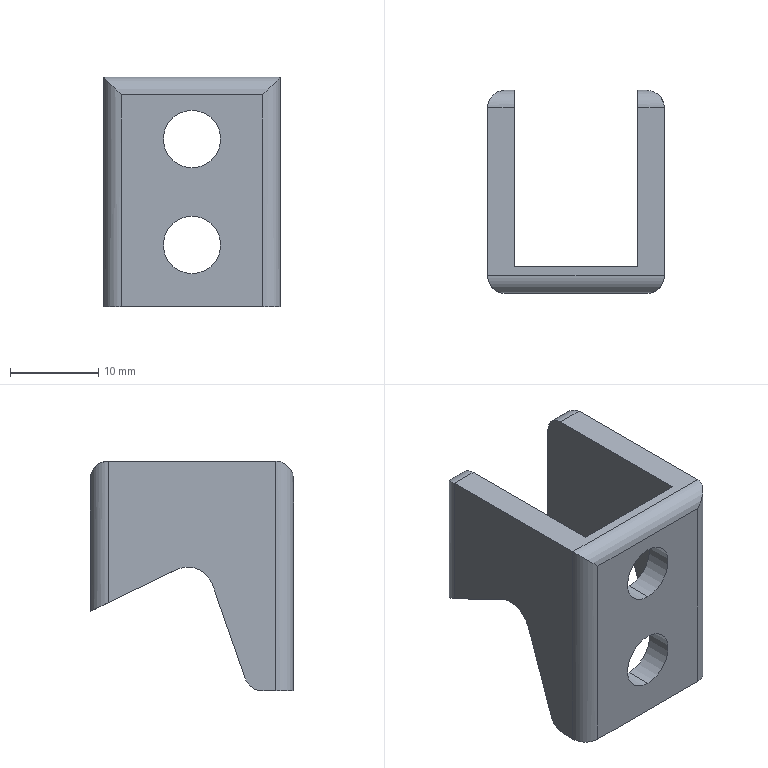Part | SolidWorks | features ICE 2, Extrusion 1, Fillet 1 | 1 solid | 31 faces | box 20 x 23 x 26 mm | volume 3238 mm3 | cylinder 17 | plane 14 | commonest cylinder face diameters 4 x9 6 x4 6.5 x4
STEP:
#1=CARTESIAN_POINT('',(0.,3.,-22.25));
#2=VERTEX_POINT('',#1);
#3=CARTESIAN_POINT('',(0.,3.,-15.75));
#4=VERTEX_POINT('',#3);
#5=CARTESIAN_POINT('',(0.,3.,-19.));
#6=DIRECTION('',(0.,1.,0.));
#7=DIRECTION('',(0.,0.,-1.));
#8=AXIS2_PLACEMENT_3D('',#5,#6,#7);
#9=CIRCLE('',#8,3.25);
#10=EDGE_CURVE('',#2,#4,#9,.T.);
#11=ORIENTED_EDGE('',*,*,#10,.T.);
#12=CARTESIAN_POINT('',(0.,0.,-15.75));
#13=VERTEX_POINT('',#12);
#14=CARTESIAN_POINT('',(0.,23.001,-15.75));
#15=DIRECTION('',(0.,-1.,0.));
#16=VECTOR('',#15,1000.);
#17=LINE('',#14,#16);
#18=EDGE_CURVE('',#4,#13,#17,.T.);
#19=ORIENTED_EDGE('',*,*,#18,.T.);
#20=CARTESIAN_POINT('',(0.,0.,-22.25));
#21=VERTEX_POINT('',#20);
#22=CARTESIAN_POINT('',(0.,0.,-19.));
#23=DIRECTION('',(0.,-1.,0.));
#24=DIRECTION('',(0.,0.,-1.));
#25=AXIS2_PLACEMENT_3D('',#22,#23,#24);
#26=CIRCLE('',#25,3.25);
#27=EDGE_CURVE('',#13,#21,#26,.T.);
#28=ORIENTED_EDGE('',*,*,#27,.T.);
#29=CARTESIAN_POINT('',(0.,23.001,-22.25));
#30=DIRECTION('',(0.,-1.,0.));
#31=VECTOR('',#30,1000.);
#32=LINE('',#29,#31);
#33=EDGE_CURVE('',#2,#21,#32,.T.);
#34=ORIENTED_EDGE('',*,*,#33,.F.);
#35=EDGE_LOOP('',(#11,#19,#28,#34));
#36=FACE_OUTER_BOUND('',#35,.T.);
#37=CARTESIAN_POINT('',(0.,23.001,-19.));
#38=DIRECTION('',(0.,-1.,0.));
#39=DIRECTION('',(0.,0.,-1.));
#40=AXIS2_PLACEMENT_3D('',#37,#38,#39);
#41=CYLINDRICAL_SURFACE('',#40,3.25);
#42=ADVANCED_FACE('',(#36),#41,.F.);
#43=CARTESIAN_POINT('',(0.,3.,-10.25));
#44=VERTEX_POINT('',#43);
#45=CARTESIAN_POINT('',(0.,3.,-3.75));
#46=VERTEX_POINT('',#45);
#47=CARTESIAN_POINT('',(0.,3.,-7.));
#48=DIRECTION('',(0.,1.,0.));
#49=DIRECTION('',(0.,0.,-1.));
#50=AXIS2_PLACEMENT_3D('',#47,#48,#49);
#51=CIRCLE('',#50,3.25);
#52=EDGE_CURVE('',#44,#46,#51,.T.);
#53=ORIENTED_EDGE('',*,*,#52,.T.);
#54=CARTESIAN_POINT('',(0.,0.,-3.75));
#55=VERTEX_POINT('',#54);
#56=CARTESIAN_POINT('',(0.,23.001,-3.75));
#57=DIRECTION('',(0.,-1.,0.));
#58=VECTOR('',#57,1000.);
#59=LINE('',#56,#58);
#60=EDGE_CURVE('',#46,#55,#59,.T.);
#61=ORIENTED_EDGE('',*,*,#60,.T.);
#62=CARTESIAN_POINT('',(0.,0.,-10.25));
#63=VERTEX_POINT('',#62);
#64=CARTESIAN_POINT('',(0.,0.,-7.));
#65=DIRECTION('',(0.,-1.,0.));
#66=DIRECTION('',(0.,0.,-1.));
#67=AXIS2_PLACEMENT_3D('',#64,#65,#66);
#68=CIRCLE('',#67,3.25);
#69=EDGE_CURVE('',#55,#63,#68,.T.);
#70=ORIENTED_EDGE('',*,*,#69,.T.);
#71=CARTESIAN_POINT('',(0.,23.001,-10.25));
#72=DIRECTION('',(0.,-1.,0.));
#73=VECTOR('',#72,1000.);
#74=LINE('',#71,#73);
#75=EDGE_CURVE('',#44,#63,#74,.T.);
#76=ORIENTED_EDGE('',*,*,#75,.F.);
#77=EDGE_LOOP('',(#53,#61,#70,#76));
#78=FACE_OUTER_BOUND('',#77,.T.);
#79=CARTESIAN_POINT('',(0.,23.001,-7.));
#80=DIRECTION('',(0.,-1.,0.));
#81=DIRECTION('',(0.,0.,-1.));
#82=AXIS2_PLACEMENT_3D('',#79,#80,#81);
#83=CYLINDRICAL_SURFACE('',#82,3.25);
#84=ADVANCED_FACE('',(#78),#83,.F.);
#85=CARTESIAN_POINT('',(10.,13.309,-12.301));
#86=VERTEX_POINT('',#85);
#87=CARTESIAN_POINT('',(10.,12.,-12.));
#88=VERTEX_POINT('',#87);
#89=CARTESIAN_POINT('',(10.,12.,-15.));
#90=DIRECTION('',(1.,0.,0.));
#91=DIRECTION('',(0.,0.,-1.));
#92=AXIS2_PLACEMENT_3D('',#89,#90,#91);
#93=CIRCLE('',#92,3.);
#94=EDGE_CURVE('',#86,#88,#93,.T.);
#95=ORIENTED_EDGE('',*,*,#94,.T.);
#96=CARTESIAN_POINT('',(7.,12.,-12.));
#97=VERTEX_POINT('',#96);
#98=CARTESIAN_POINT('',(10.,12.,-12.));
#99=DIRECTION('',(-1.,0.,0.));
#100=VECTOR('',#99,1000.);
#101=LINE('',#98,#100);
#102=EDGE_CURVE('',#88,#97,#101,.T.);
#103=ORIENTED_EDGE('',*,*,#102,.T.);
#104=CARTESIAN_POINT('',(7.,13.309,-12.301));
#105=VERTEX_POINT('',#104);
#106=CARTESIAN_POINT('',(7.,12.,-15.));
#107=DIRECTION('',(1.,0.,0.));
#108=DIRECTION('',(0.,0.,-1.));
#109=AXIS2_PLACEMENT_3D('',#106,#107,#108);
#110=CIRCLE('',#109,3.);
#111=EDGE_CURVE('',#105,#97,#110,.T.);
#112=ORIENTED_EDGE('',*,*,#111,.F.);
#113=CARTESIAN_POINT('',(10.,13.309,-12.301));
#114=DIRECTION('',(-1.,0.,0.));
#115=VECTOR('',#114,1000.);
#116=LINE('',#113,#115);
#117=EDGE_CURVE('',#86,#105,#116,.T.);
#118=ORIENTED_EDGE('',*,*,#117,.F.);
#119=EDGE_LOOP('',(#95,#103,#112,#118));
#120=FACE_OUTER_BOUND('',#119,.T.);
#121=CARTESIAN_POINT('',(10.,12.,-15.));
#122=DIRECTION('',(-1.,0.,0.));
#123=DIRECTION('',(0.,0.,1.));
#124=AXIS2_PLACEMENT_3D('',#121,#122,#123);
#125=CYLINDRICAL_SURFACE('',#124,3.);
#126=ADVANCED_FACE('',(#120),#125,.F.);
#127=CARTESIAN_POINT('',(-7.,13.309,-12.301));
#128=VERTEX_POINT('',#127);
#129=CARTESIAN_POINT('',(-7.,12.,-12.));
#130=VERTEX_POINT('',#129);
#131=CARTESIAN_POINT('',(-7.,12.,-15.));
#132=DIRECTION('',(1.,0.,0.));
#133=DIRECTION('',(0.,0.,-1.));
#134=AXIS2_PLACEMENT_3D('',#131,#132,#133);
#135=CIRCLE('',#134,3.);
#136=EDGE_CURVE('',#128,#130,#135,.T.);
#137=ORIENTED_EDGE('',*,*,#136,.T.);
#138=CARTESIAN_POINT('',(-10.,12.,-12.));
#139=VERTEX_POINT('',#138);
#140=CARTESIAN_POINT('',(10.,12.,-12.));
#141=DIRECTION('',(-1.,0.,0.));
#142=VECTOR('',#141,1000.);
#143=LINE('',#140,#142);
#144=EDGE_CURVE('',#130,#139,#143,.T.);
#145=ORIENTED_EDGE('',*,*,#144,.T.);
#146=CARTESIAN_POINT('',(-10.,13.309,-12.301));
#147=VERTEX_POINT('',#146);
#148=CARTESIAN_POINT('',(-10.,12.,-15.));
#149=DIRECTION('',(1.,0.,0.));
#150=DIRECTION('',(0.,0.,-1.));
#151=AXIS2_PLACEMENT_3D('',#148,#149,#150);
#152=CIRCLE('',#151,3.);
#153=EDGE_CURVE('',#147,#139,#152,.T.);
#154=ORIENTED_EDGE('',*,*,#153,.F.);
#155=CARTESIAN_POINT('',(10.,13.309,-12.301));
#156=DIRECTION('',(-1.,0.,0.));
#157=VECTOR('',#156,1000.);
#158=LINE('',#155,#157);
#159=EDGE_CURVE('',#128,#147,#158,.T.);
#160=ORIENTED_EDGE('',*,*,#159,.F.);
#161=EDGE_LOOP('',(#137,#145,#154,#160));
#162=FACE_OUTER_BOUND('',#161,.T.);
#163=CARTESIAN_POINT('',(10.,12.,-15.));
#164=DIRECTION('',(-1.,0.,0.));
#165=DIRECTION('',(0.,0.,1.));
#166=AXIS2_PLACEMENT_3D('',#163,#164,#165);
#167=CYLINDRICAL_SURFACE('',#166,3.);
#168=ADVANCED_FACE('',(#162),#167,.F.);
#169=ORIENTED_EDGE('',*,*,#144,.F.);
#170=CARTESIAN_POINT('',(-7.,9.166,-14.015));
#171=VERTEX_POINT('',#170);
#172=CARTESIAN_POINT('',(-7.,12.,-15.));
#173=DIRECTION('',(1.,0.,0.));
#174=DIRECTION('',(0.,0.,-1.));
#175=AXIS2_PLACEMENT_3D('',#172,#173,#174);
#176=CIRCLE('',#175,3.);
#177=EDGE_CURVE('',#130,#171,#176,.T.);
#178=ORIENTED_EDGE('',*,*,#177,.T.);
#179=CARTESIAN_POINT('',(-10.,9.166,-14.015));
#180=VERTEX_POINT('',#179);
#181=CARTESIAN_POINT('',(10.,9.166,-14.015));
#182=DIRECTION('',(-1.,0.,0.));
#183=VECTOR('',#182,1000.);
#184=LINE('',#181,#183);
#185=EDGE_CURVE('',#171,#180,#184,.T.);
#186=ORIENTED_EDGE('',*,*,#185,.T.);
#187=CARTESIAN_POINT('',(-10.,12.,-15.));
#188=DIRECTION('',(1.,0.,0.));
#189=DIRECTION('',(0.,0.,-1.));
#190=AXIS2_PLACEMENT_3D('',#187,#188,#189);
#191=CIRCLE('',#190,3.);
#192=EDGE_CURVE('',#139,#180,#191,.T.);
#193=ORIENTED_EDGE('',*,*,#192,.F.);
#194=EDGE_LOOP('',(#169,#178,#186,#193));
#195=FACE_OUTER_BOUND('',#194,.T.);
#196=CARTESIAN_POINT('',(10.,12.,-15.));
#197=DIRECTION('',(-1.,0.,0.));
#198=DIRECTION('',(0.,0.,1.));
#199=AXIS2_PLACEMENT_3D('',#196,#197,#198);
#200=CYLINDRICAL_SURFACE('',#199,3.);
#201=ADVANCED_FACE('',(#195),#200,.F.);
#202=CARTESIAN_POINT('',(-10.,21.,-16.03));
#203=VERTEX_POINT('',#202);
#204=CARTESIAN_POINT('',(-10.,-2.295,-4.734));
#205=DIRECTION('',(0.,-0.8998,0.4363));
#206=VECTOR('',#205,1000.);
#207=LINE('',#204,#206);
#208=EDGE_CURVE('',#203,#147,#207,.T.);
#209=ORIENTED_EDGE('',*,*,#208,.F.);
#210=CARTESIAN_POINT('',(-8.,23.,-17.));
#211=VERTEX_POINT('',#210);
#212=CARTESIAN_POINT('',(-10.,21.,-16.03));
#213=CARTESIAN_POINT('',(-10.,22.172,-16.598));
#214=CARTESIAN_POINT('',(-9.172,23.,-17.));
#215=CARTESIAN_POINT('',(-8.,23.,-17.));
#216=(BOUNDED_CURVE()B_SPLINE_CURVE(3,(#212,#213,#214,#215),.UNSPECIFIED.,.F.,.T.)B_SPLINE_CURVE_WITH_KNOTS((4,4),(1.571,3.142),.UNSPECIFIED.)CURVE()GEOMETRIC_REPRESENTATION_ITEM()RATIONAL_B_SPLINE_CURVE((1.,0.8047,0.8047,1.))REPRESENTATION_ITEM(''));
#217=EDGE_CURVE('',#203,#211,#216,.T.);
#218=ORIENTED_EDGE('',*,*,#217,.T.);
#219=CARTESIAN_POINT('',(-7.,23.,-17.));
#220=VERTEX_POINT('',#219);
#221=CARTESIAN_POINT('',(10.,23.,-17.));
#222=DIRECTION('',(-1.,0.,0.));
#223=VECTOR('',#222,1000.);
#224=LINE('',#221,#223);
#225=EDGE_CURVE('',#220,#211,#224,.T.);
#226=ORIENTED_EDGE('',*,*,#225,.F.);
#227=CARTESIAN_POINT('',(-7.,-2.295,-4.734));
#228=DIRECTION('',(0.,-0.8998,0.4363));
#229=VECTOR('',#228,1000.);
#230=LINE('',#227,#229);
#231=EDGE_CURVE('',#220,#128,#230,.T.);
#232=ORIENTED_EDGE('',*,*,#231,.T.);
#233=ORIENTED_EDGE('',*,*,#159,.T.);
#234=EDGE_LOOP('',(#209,#218,#226,#232,#233));
#235=FACE_OUTER_BOUND('',#234,.T.);
#236=CARTESIAN_POINT('',(10.,-2.295,-4.734));
#237=DIRECTION('',(0.,-0.4363,-0.8998));
#238=DIRECTION('',(0.,0.8998,-0.4363));
#239=AXIS2_PLACEMENT_3D('',#236,#237,#238);
#240=PLANE('',#239);
#241=ADVANCED_FACE('',(#235),#240,.T.);
#242=ORIENTED_EDGE('',*,*,#225,.T.);
#243=CARTESIAN_POINT('',(-8.,23.,-2.));
#244=VERTEX_POINT('',#243);
#245=CARTESIAN_POINT('',(-8.,23.,0.));
#246=DIRECTION('',(0.,0.,1.));
#247=VECTOR('',#246,1000.);
#248=LINE('',#245,#247);
#249=EDGE_CURVE('',#211,#244,#248,.T.);
#250=ORIENTED_EDGE('',*,*,#249,.T.);
#251=CARTESIAN_POINT('',(-7.,23.,-2.));
#252=VERTEX_POINT('',#251);
#253=CARTESIAN_POINT('',(-7.,23.,-2.));
#254=DIRECTION('',(1.,0.,0.));
#255=VECTOR('',#254,1000.);
#256=LINE('',#253,#255);
#257=EDGE_CURVE('',#244,#252,#256,.T.);
#258=ORIENTED_EDGE('',*,*,#257,.T.);
#259=CARTESIAN_POINT('',(-7.,23.,0.));
#260=DIRECTION('',(0.,0.,1.));
#261=VECTOR('',#260,1000.);
#262=LINE('',#259,#261);
#263=EDGE_CURVE('',#220,#252,#262,.T.);
#264=ORIENTED_EDGE('',*,*,#263,.F.);
#265=EDGE_LOOP('',(#242,#250,#258,#264));
#266=FACE_OUTER_BOUND('',#265,.T.);
#267=CARTESIAN_POINT('',(10.,23.,0.));
#268=DIRECTION('',(0.,1.,0.));
#269=DIRECTION('',(0.,0.,1.));
#270=AXIS2_PLACEMENT_3D('',#267,#268,#269);
#271=PLANE('',#270);
#272=ADVANCED_FACE('',(#266),#271,.T.);
#273=CARTESIAN_POINT('',(-10.,21.,0.));
#274=VERTEX_POINT('',#273);
#275=CARTESIAN_POINT('',(-10.,2.,0.));
#276=VERTEX_POINT('',#275);
#277=CARTESIAN_POINT('',(-10.,0.,0.));
#278=DIRECTION('',(0.,-1.,0.));
#279=VECTOR('',#278,1000.);
#280=LINE('',#277,#279);
#281=EDGE_CURVE('',#274,#276,#280,.T.);
#282=ORIENTED_EDGE('',*,*,#281,.T.);
#283=CARTESIAN_POINT('',(10.,2.,0.));
#284=VERTEX_POINT('',#283);
#285=CARTESIAN_POINT('',(10.,2.,0.));
#286=DIRECTION('',(1.,0.,0.));
#287=VECTOR('',#286,1000.);
#288=LINE('',#285,#287);
#289=EDGE_CURVE('',#276,#284,#288,.T.);
#290=ORIENTED_EDGE('',*,*,#289,.T.);
#291=CARTESIAN_POINT('',(10.,21.,0.));
#292=VERTEX_POINT('',#291);
#293=CARTESIAN_POINT('',(10.,0.,0.));
#294=DIRECTION('',(0.,-1.,0.));
#295=VECTOR('',#294,1000.);
#296=LINE('',#293,#295);
#297=EDGE_CURVE('',#292,#284,#296,.T.);
#298=ORIENTED_EDGE('',*,*,#297,.F.);
#299=CARTESIAN_POINT('',(7.,21.,0.));
#300=VERTEX_POINT('',#299);
#301=CARTESIAN_POINT('',(7.,21.,0.));
#302=DIRECTION('',(-1.,0.,0.));
#303=VECTOR('',#302,1000.);
#304=LINE('',#301,#303);
#305=EDGE_CURVE('',#292,#300,#304,.T.);
#306=ORIENTED_EDGE('',*,*,#305,.T.);
#307=CARTESIAN_POINT('',(7.,3.,0.));
#308=VERTEX_POINT('',#307);
#309=CARTESIAN_POINT('',(7.,23.,0.));
#310=DIRECTION('',(0.,-1.,0.));
#311=VECTOR('',#310,1000.);
#312=LINE('',#309,#311);
#313=EDGE_CURVE('',#300,#308,#312,.T.);
#314=ORIENTED_EDGE('',*,*,#313,.T.);
#315=CARTESIAN_POINT('',(-7.,3.,0.));
#316=VERTEX_POINT('',#315);
#317=CARTESIAN_POINT('',(-7.,3.,0.));
#318=DIRECTION('',(1.,0.,0.));
#319=VECTOR('',#318,1000.);
#320=LINE('',#317,#319);
#321=EDGE_CURVE('',#316,#308,#320,.T.);
#322=ORIENTED_EDGE('',*,*,#321,.F.);
#323=CARTESIAN_POINT('',(-7.,21.,0.));
#324=VERTEX_POINT('',#323);
#325=CARTESIAN_POINT('',(-7.,23.,0.));
#326=DIRECTION('',(0.,-1.,0.));
#327=VECTOR('',#326,1000.);
#328=LINE('',#325,#327);
#329=EDGE_CURVE('',#324,#316,#328,.T.);
#330=ORIENTED_EDGE('',*,*,#329,.F.);
#331=CARTESIAN_POINT('',(-10.,21.,0.));
#332=DIRECTION('',(-1.,0.,0.));
#333=VECTOR('',#332,1000.);
#334=LINE('',#331,#333);
#335=EDGE_CURVE('',#324,#274,#334,.T.);
#336=ORIENTED_EDGE('',*,*,#335,.T.);
#337=EDGE_LOOP('',(#282,#290,#298,#306,#314,#322,#330,#336));
#338=FACE_OUTER_BOUND('',#337,.T.);
#339=CARTESIAN_POINT('',(10.,0.,0.));
#340=DIRECTION('',(0.,0.,-1.));
#341=DIRECTION('',(0.,1.,0.));
#342=AXIS2_PLACEMENT_3D('',#339,#340,#341);
#343=PLANE('',#342);
#344=ADVANCED_FACE('',(#338),#343,.F.);
#345=CARTESIAN_POINT('',(7.,3.,-26.));
#346=VERTEX_POINT('',#345);
#347=CARTESIAN_POINT('',(7.,3.578,-26.));
#348=VERTEX_POINT('',#347);
#349=CARTESIAN_POINT('',(7.,23.,-26.));
#350=DIRECTION('',(0.,1.,0.));
#351=VECTOR('',#350,1000.);
#352=LINE('',#349,#351);
#353=EDGE_CURVE('',#346,#348,#352,.T.);
#354=ORIENTED_EDGE('',*,*,#353,.T.);
#355=CARTESIAN_POINT('',(10.,3.578,-26.));
#356=VERTEX_POINT('',#355);
#357=CARTESIAN_POINT('',(10.,3.578,-26.));
#358=DIRECTION('',(1.,0.,0.));
#359=VECTOR('',#358,1000.);
#360=LINE('',#357,#359);
#361=EDGE_CURVE('',#348,#356,#360,.T.);
#362=ORIENTED_EDGE('',*,*,#361,.T.);
#363=CARTESIAN_POINT('',(10.,2.,-26.));
#364=VERTEX_POINT('',#363);
#365=CARTESIAN_POINT('',(10.,0.,-26.));
#366=DIRECTION('',(0.,1.,0.));
#367=VECTOR('',#366,1000.);
#368=LINE('',#365,#367);
#369=EDGE_CURVE('',#364,#356,#368,.T.);
#370=ORIENTED_EDGE('',*,*,#369,.F.);
#371=CARTESIAN_POINT('',(8.,0.,-26.));
#372=VERTEX_POINT('',#371);
#373=CARTESIAN_POINT('',(8.,2.,-26.));
#374=DIRECTION('',(0.,0.,-1.));
#375=DIRECTION('',(1.,0.,0.));
#376=AXIS2_PLACEMENT_3D('',#373,#374,#375);
#377=CIRCLE('',#376,2.);
#378=EDGE_CURVE('',#364,#372,#377,.T.);
#379=ORIENTED_EDGE('',*,*,#378,.T.);
#380=CARTESIAN_POINT('',(-8.,0.,-26.));
#381=VERTEX_POINT('',#380);
#382=CARTESIAN_POINT('',(10.,0.,-26.));
#383=DIRECTION('',(-1.,0.,0.));
#384=VECTOR('',#383,1000.);
#385=LINE('',#382,#384);
#386=EDGE_CURVE('',#372,#381,#385,.T.);
#387=ORIENTED_EDGE('',*,*,#386,.T.);
#388=CARTESIAN_POINT('',(-10.,2.,-26.));
#389=VERTEX_POINT('',#388);
#390=CARTESIAN_POINT('',(-8.,2.,-26.));
#391=DIRECTION('',(0.,0.,-1.));
#392=DIRECTION('',(1.,0.,0.));
#393=AXIS2_PLACEMENT_3D('',#390,#391,#392);
#394=CIRCLE('',#393,2.);
#395=EDGE_CURVE('',#381,#389,#394,.T.);
#396=ORIENTED_EDGE('',*,*,#395,.T.);
#397=CARTESIAN_POINT('',(-10.,3.578,-26.));
#398=VERTEX_POINT('',#397);
#399=CARTESIAN_POINT('',(-10.,0.,-26.));
#400=DIRECTION('',(0.,1.,0.));
#401=VECTOR('',#400,1000.);
#402=LINE('',#399,#401);
#403=EDGE_CURVE('',#389,#398,#402,.T.);
#404=ORIENTED_EDGE('',*,*,#403,.T.);
#405=CARTESIAN_POINT('',(-7.,3.578,-26.));
#406=VERTEX_POINT('',#405);
#407=CARTESIAN_POINT('',(10.,3.578,-26.));
#408=DIRECTION('',(1.,0.,0.));
#409=VECTOR('',#408,1000.);
#410=LINE('',#407,#409);
#411=EDGE_CURVE('',#398,#406,#410,.T.);
#412=ORIENTED_EDGE('',*,*,#411,.T.);
#413=CARTESIAN_POINT('',(-7.,3.,-26.));
#414=VERTEX_POINT('',#413);
#415=CARTESIAN_POINT('',(-7.,23.,-26.));
#416=DIRECTION('',(0.,1.,0.));
#417=VECTOR('',#416,1000.);
#418=LINE('',#415,#417);
#419=EDGE_CURVE('',#414,#406,#418,.T.);
#420=ORIENTED_EDGE('',*,*,#419,.F.);
#421=CARTESIAN_POINT('',(-7.,3.,-26.));
#422=DIRECTION('',(1.,0.,0.));
#423=VECTOR('',#422,1000.);
#424=LINE('',#421,#423);
#425=EDGE_CURVE('',#414,#346,#424,.T.);
#426=ORIENTED_EDGE('',*,*,#425,.T.);
#427=EDGE_LOOP('',(#354,#362,#370,#379,#387,#396,#404,#412,#420,#426));
#428=FACE_OUTER_BOUND('',#427,.T.);
#429=CARTESIAN_POINT('',(10.,0.,-26.));
#430=DIRECTION('',(0.,0.,1.));
#431=DIRECTION('',(1.,0.,0.));
#432=AXIS2_PLACEMENT_3D('',#429,#430,#431);
#433=PLANE('',#432);
#434=ADVANCED_FACE('',(#428),#433,.F.);
#435=CARTESIAN_POINT('',(-7.,5.467,-24.657));
#436=VERTEX_POINT('',#435);
#437=CARTESIAN_POINT('',(-7.,12.525,-4.354));
#438=DIRECTION('',(0.,0.3284,0.9446));
#439=VECTOR('',#438,1000.);
#440=LINE('',#437,#439);
#441=EDGE_CURVE('',#436,#171,#440,.T.);
#442=ORIENTED_EDGE('',*,*,#441,.F.);
#443=CARTESIAN_POINT('',(-10.,5.467,-24.657));
#444=VERTEX_POINT('',#443);
#445=CARTESIAN_POINT('',(10.,5.467,-24.657));
#446=DIRECTION('',(-1.,0.,0.));
#447=VECTOR('',#446,1000.);
#448=LINE('',#445,#447);
#449=EDGE_CURVE('',#436,#444,#448,.T.);
#450=ORIENTED_EDGE('',*,*,#449,.T.);
#451=CARTESIAN_POINT('',(-10.,12.525,-4.354));
#452=DIRECTION('',(0.,0.3284,0.9446));
#453=VECTOR('',#452,1000.);
#454=LINE('',#451,#453);
#455=EDGE_CURVE('',#444,#180,#454,.T.);
#456=ORIENTED_EDGE('',*,*,#455,.T.);
#457=ORIENTED_EDGE('',*,*,#185,.F.);
#458=EDGE_LOOP('',(#442,#450,#456,#457));
#459=FACE_OUTER_BOUND('',#458,.T.);
#460=CARTESIAN_POINT('',(10.,12.525,-4.354));
#461=DIRECTION('',(0.,-0.9446,0.3284));
#462=DIRECTION('',(0.,-0.3284,-0.9446));
#463=AXIS2_PLACEMENT_3D('',#460,#461,#462);
#464=PLANE('',#463);
#465=ADVANCED_FACE('',(#459),#464,.F.);
#466=ORIENTED_EDGE('',*,*,#102,.F.);
#467=CARTESIAN_POINT('',(10.,9.166,-14.015));
#468=VERTEX_POINT('',#467);
#469=CARTESIAN_POINT('',(10.,12.,-15.));
#470=DIRECTION('',(1.,0.,0.));
#471=DIRECTION('',(0.,0.,-1.));
#472=AXIS2_PLACEMENT_3D('',#469,#470,#471);
#473=CIRCLE('',#472,3.);
#474=EDGE_CURVE('',#88,#468,#473,.T.);
#475=ORIENTED_EDGE('',*,*,#474,.T.);
#476=CARTESIAN_POINT('',(7.,9.166,-14.015));
#477=VERTEX_POINT('',#476);
#478=CARTESIAN_POINT('',(10.,9.166,-14.015));
#479=DIRECTION('',(-1.,0.,0.));
#480=VECTOR('',#479,1000.);
#481=LINE('',#478,#480);
#482=EDGE_CURVE('',#468,#477,#481,.T.);
#483=ORIENTED_EDGE('',*,*,#482,.T.);
#484=CARTESIAN_POINT('',(7.,12.,-15.));
#485=DIRECTION('',(1.,0.,0.));
#486=DIRECTION('',(0.,0.,-1.));
#487=AXIS2_PLACEMENT_3D('',#484,#485,#486);
#488=CIRCLE('',#487,3.);
#489=EDGE_CURVE('',#97,#477,#488,.T.);
#490=ORIENTED_EDGE('',*,*,#489,.F.);
#491=EDGE_LOOP('',(#466,#475,#483,#490));
#492=FACE_OUTER_BOUND('',#491,.T.);
#493=CARTESIAN_POINT('',(10.,12.,-15.));
#494=DIRECTION('',(-1.,0.,0.));
#495=DIRECTION('',(0.,0.,1.));
#496=AXIS2_PLACEMENT_3D('',#493,#494,#495);
#497=CYLINDRICAL_SURFACE('',#496,3.);
#498=ADVANCED_FACE('',(#492),#497,.F.);
#499=CARTESIAN_POINT('',(8.,23.,-17.));
#500=VERTEX_POINT('',#499);
#501=CARTESIAN_POINT('',(7.,23.,-17.));
#502=VERTEX_POINT('',#501);
#503=CARTESIAN_POINT('',(10.,23.,-17.));
#504=DIRECTION('',(-1.,0.,0.));
#505=VECTOR('',#504,1000.);
#506=LINE('',#503,#505);
#507=EDGE_CURVE('',#500,#502,#506,.T.);
#508=ORIENTED_EDGE('',*,*,#507,.F.);
#509=CARTESIAN_POINT('',(10.,21.,-16.03));
#510=VERTEX_POINT('',#509);
#511=CARTESIAN_POINT('',(8.,23.,-17.));
#512=CARTESIAN_POINT('',(9.172,23.,-17.));
#513=CARTESIAN_POINT('',(10.,22.172,-16.598));
#514=CARTESIAN_POINT('',(10.,21.,-16.03));
#515=(BOUNDED_CURVE()B_SPLINE_CURVE(3,(#511,#512,#513,#514),.UNSPECIFIED.,.F.,.F.)B_SPLINE_CURVE_WITH_KNOTS((4,4),(0.,1.571),.UNSPECIFIED.)CURVE()GEOMETRIC_REPRESENTATION_ITEM()RATIONAL_B_SPLINE_CURVE((1.,0.8047,0.8047,1.))REPRESENTATION_ITEM(''));
#516=EDGE_CURVE('',#500,#510,#515,.T.);
#517=ORIENTED_EDGE('',*,*,#516,.T.);
#518=CARTESIAN_POINT('',(10.,-2.295,-4.734));
#519=DIRECTION('',(0.,-0.8998,0.4363));
#520=VECTOR('',#519,1000.);
#521=LINE('',#518,#520);
#522=EDGE_CURVE('',#510,#86,#521,.T.);
#523=ORIENTED_EDGE('',*,*,#522,.T.);
#524=ORIENTED_EDGE('',*,*,#117,.T.);
#525=CARTESIAN_POINT('',(7.,-2.295,-4.734));
#526=DIRECTION('',(0.,-0.8998,0.4363));
#527=VECTOR('',#526,1000.);
#528=LINE('',#525,#527);
#529=EDGE_CURVE('',#502,#105,#528,.T.);
#530=ORIENTED_EDGE('',*,*,#529,.F.);
#531=EDGE_LOOP('',(#508,#517,#523,#524,#530));
#532=FACE_OUTER_BOUND('',#531,.T.);
#533=CARTESIAN_POINT('',(10.,-2.295,-4.734));
#534=DIRECTION('',(0.,-0.4363,-0.8998));
#535=DIRECTION('',(0.,0.8998,-0.4363));
#536=AXIS2_PLACEMENT_3D('',#533,#534,#535);
#537=PLANE('',#536);
#538=ADVANCED_FACE('',(#532),#537,.T.);
#539=CARTESIAN_POINT('',(7.,23.,-2.));
#540=VERTEX_POINT('',#539);
#541=CARTESIAN_POINT('',(8.,23.,-2.));
#542=VERTEX_POINT('',#541);
#543=CARTESIAN_POINT('',(10.,23.,-2.));
#544=DIRECTION('',(1.,0.,0.));
#545=VECTOR('',#544,1000.);
#546=LINE('',#543,#545);
#547=EDGE_CURVE('',#540,#542,#546,.T.);
#548=ORIENTED_EDGE('',*,*,#547,.T.);
#549=CARTESIAN_POINT('',(8.,23.,0.));
#550=DIRECTION('',(0.,0.,-1.));
#551=VECTOR('',#550,1000.);
#552=LINE('',#549,#551);
#553=EDGE_CURVE('',#542,#500,#552,.T.);
#554=ORIENTED_EDGE('',*,*,#553,.T.);
#555=ORIENTED_EDGE('',*,*,#507,.T.);
#556=CARTESIAN_POINT('',(7.,23.,0.));
#557=DIRECTION('',(0.,0.,1.));
#558=VECTOR('',#557,1000.);
#559=LINE('',#556,#558);
#560=EDGE_CURVE('',#502,#540,#559,.T.);
#561=ORIENTED_EDGE('',*,*,#560,.T.);
#562=EDGE_LOOP('',(#548,#554,#555,#561));
#563=FACE_OUTER_BOUND('',#562,.T.);
#564=CARTESIAN_POINT('',(10.,23.,0.));
#565=DIRECTION('',(0.,1.,0.));
#566=DIRECTION('',(0.,0.,1.));
#567=AXIS2_PLACEMENT_3D('',#564,#565,#566);
#568=PLANE('',#567);
#569=ADVANCED_FACE('',(#563),#568,.T.);
#570=CARTESIAN_POINT('',(0.,0.,-19.));
#571=DIRECTION('',(0.,-1.,0.));
#572=DIRECTION('',(0.,0.,-1.));
#573=AXIS2_PLACEMENT_3D('',#570,#571,#572);
#574=CIRCLE('',#573,3.25);
#575=EDGE_CURVE('',#21,#13,#574,.T.);
#576=ORIENTED_EDGE('',*,*,#575,.F.);
#577=ORIENTED_EDGE('',*,*,#27,.F.);
#578=EDGE_LOOP('',(#576,#577));
#579=FACE_BOUND('',#578,.T.);
#580=CARTESIAN_POINT('',(0.,0.,-7.));
#581=DIRECTION('',(0.,-1.,0.));
#582=DIRECTION('',(0.,0.,-1.));
#583=AXIS2_PLACEMENT_3D('',#580,#581,#582);
#584=CIRCLE('',#583,3.25);
#585=EDGE_CURVE('',#63,#55,#584,.T.);
#586=ORIENTED_EDGE('',*,*,#585,.F.);
#587=ORIENTED_EDGE('',*,*,#69,.F.);
#588=EDGE_LOOP('',(#586,#587));
#589=FACE_BOUND('',#588,.T.);
#590=CARTESIAN_POINT('',(8.,0.,-2.));
#591=VERTEX_POINT('',#590);
#592=CARTESIAN_POINT('',(-8.,0.,-2.));
#593=VERTEX_POINT('',#592);
#594=CARTESIAN_POINT('',(10.,0.,-2.));
#595=DIRECTION('',(-1.,0.,0.));
#596=VECTOR('',#595,1000.);
#597=LINE('',#594,#596);
#598=EDGE_CURVE('',#591,#593,#597,.T.);
#599=ORIENTED_EDGE('',*,*,#598,.T.);
#600=CARTESIAN_POINT('',(-8.,0.,0.));
#601=DIRECTION('',(0.,0.,-1.));
#602=VECTOR('',#601,1000.);
#603=LINE('',#600,#602);
#604=EDGE_CURVE('',#593,#381,#603,.T.);
#605=ORIENTED_EDGE('',*,*,#604,.T.);
#606=ORIENTED_EDGE('',*,*,#386,.F.);
#607=CARTESIAN_POINT('',(8.,0.,0.));
#608=DIRECTION('',(0.,0.,1.));
#609=VECTOR('',#608,1000.);
#610=LINE('',#607,#609);
#611=EDGE_CURVE('',#372,#591,#610,.T.);
#612=ORIENTED_EDGE('',*,*,#611,.T.);
#613=EDGE_LOOP('',(#599,#605,#606,#612));
#614=FACE_OUTER_BOUND('',#613,.T.);
#615=CARTESIAN_POINT('',(10.,0.,0.));
#616=DIRECTION('',(0.,1.,0.));
#617=DIRECTION('',(0.,0.,1.));
#618=AXIS2_PLACEMENT_3D('',#615,#616,#617);
#619=PLANE('',#618);
#620=ADVANCED_FACE('',(#579,#589,#614),#619,.F.);
#621=CARTESIAN_POINT('',(10.,5.467,-24.657));
#622=VERTEX_POINT('',#621);
#623=CARTESIAN_POINT('',(10.,12.525,-4.354));
#624=DIRECTION('',(0.,0.3284,0.9446));
#625=VECTOR('',#624,1000.);
#626=LINE('',#623,#625);
#627=EDGE_CURVE('',#622,#468,#626,.T.);
#628=ORIENTED_EDGE('',*,*,#627,.F.);
#629=CARTESIAN_POINT('',(7.,5.467,-24.657));
#630=VERTEX_POINT('',#629);
#631=CARTESIAN_POINT('',(10.,5.467,-24.657));
#632=DIRECTION('',(-1.,0.,0.));
#633=VECTOR('',#632,1000.);
#634=LINE('',#631,#633);
#635=EDGE_CURVE('',#622,#630,#634,.T.);
#636=ORIENTED_EDGE('',*,*,#635,.T.);
#637=CARTESIAN_POINT('',(7.,12.525,-4.354));
#638=DIRECTION('',(0.,0.3284,0.9446));
#639=VECTOR('',#638,1000.);
#640=LINE('',#637,#639);
#641=EDGE_CURVE('',#630,#477,#640,.T.);
#642=ORIENTED_EDGE('',*,*,#641,.T.);
#643=ORIENTED_EDGE('',*,*,#482,.F.);
#644=EDGE_LOOP('',(#628,#636,#642,#643));
#645=FACE_OUTER_BOUND('',#644,.T.);
#646=CARTESIAN_POINT('',(10.,12.525,-4.354));
#647=DIRECTION('',(0.,-0.9446,0.3284));
#648=DIRECTION('',(0.,-0.3284,-0.9446));
#649=AXIS2_PLACEMENT_3D('',#646,#647,#648);
#650=PLANE('',#649);
#651=ADVANCED_FACE('',(#645),#650,.F.);
#652=ORIENTED_EDGE('',*,*,#369,.T.);
#653=CARTESIAN_POINT('',(10.,3.578,-24.));
#654=DIRECTION('',(1.,0.,0.));
#655=DIRECTION('',(0.,0.,-1.));
#656=AXIS2_PLACEMENT_3D('',#653,#654,#655);
#657=CIRCLE('',#656,2.);
#658=EDGE_CURVE('',#356,#622,#657,.T.);
#659=ORIENTED_EDGE('',*,*,#658,.T.);
#660=ORIENTED_EDGE('',*,*,#627,.T.);
#661=ORIENTED_EDGE('',*,*,#474,.F.);
#662=ORIENTED_EDGE('',*,*,#94,.F.);
#663=ORIENTED_EDGE('',*,*,#522,.F.);
#664=CARTESIAN_POINT('',(10.,21.,0.));
#665=DIRECTION('',(0.,0.,1.));
#666=VECTOR('',#665,1000.);
#667=LINE('',#664,#666);
#668=EDGE_CURVE('',#510,#292,#667,.T.);
#669=ORIENTED_EDGE('',*,*,#668,.T.);
#670=ORIENTED_EDGE('',*,*,#297,.T.);
#671=CARTESIAN_POINT('',(10.,2.,-26.));
#672=DIRECTION('',(0.,0.,-1.));
#673=VECTOR('',#672,1000.);
#674=LINE('',#671,#673);
#675=EDGE_CURVE('',#284,#364,#674,.T.);
#676=ORIENTED_EDGE('',*,*,#675,.T.);
#677=EDGE_LOOP('',(#652,#659,#660,#661,#662,#663,#669,#670,#676));
#678=FACE_OUTER_BOUND('',#677,.T.);
#679=CARTESIAN_POINT('',(10.,0.,0.));
#680=DIRECTION('',(1.,0.,0.));
#681=DIRECTION('',(0.,0.,-1.));
#682=AXIS2_PLACEMENT_3D('',#679,#680,#681);
#683=PLANE('',#682);
#684=ADVANCED_FACE('',(#678),#683,.T.);
#685=ORIENTED_EDGE('',*,*,#455,.F.);
#686=CARTESIAN_POINT('',(-10.,3.578,-24.));
#687=DIRECTION('',(-1.,0.,0.));
#688=DIRECTION('',(0.,0.,-1.));
#689=AXIS2_PLACEMENT_3D('',#686,#687,#688);
#690=CIRCLE('',#689,2.);
#691=EDGE_CURVE('',#444,#398,#690,.T.);
#692=ORIENTED_EDGE('',*,*,#691,.T.);
#693=ORIENTED_EDGE('',*,*,#403,.F.);
#694=CARTESIAN_POINT('',(-10.,2.,0.));
#695=DIRECTION('',(0.,0.,1.));
#696=VECTOR('',#695,1000.);
#697=LINE('',#694,#696);
#698=EDGE_CURVE('',#389,#276,#697,.T.);
#699=ORIENTED_EDGE('',*,*,#698,.T.);
#700=ORIENTED_EDGE('',*,*,#281,.F.);
#701=CARTESIAN_POINT('',(-10.,21.,-17.));
#702=DIRECTION('',(0.,0.,-1.));
#703=VECTOR('',#702,1000.);
#704=LINE('',#701,#703);
#705=EDGE_CURVE('',#274,#203,#704,.T.);
#706=ORIENTED_EDGE('',*,*,#705,.T.);
#707=ORIENTED_EDGE('',*,*,#208,.T.);
#708=ORIENTED_EDGE('',*,*,#153,.T.);
#709=ORIENTED_EDGE('',*,*,#192,.T.);
#710=EDGE_LOOP('',(#685,#692,#693,#699,#700,#706,#707,#708,#709));
#711=FACE_OUTER_BOUND('',#710,.T.);
#712=CARTESIAN_POINT('',(-10.,0.,0.));
#713=DIRECTION('',(1.,0.,0.));
#714=DIRECTION('',(0.,0.,-1.));
#715=AXIS2_PLACEMENT_3D('',#712,#713,#714);
#716=PLANE('',#715);
#717=ADVANCED_FACE('',(#711),#716,.F.);
#718=ORIENTED_EDGE('',*,*,#10,.F.);
#719=CARTESIAN_POINT('',(0.,3.,-19.));
#720=DIRECTION('',(0.,1.,0.));
#721=DIRECTION('',(0.,0.,-1.));
#722=AXIS2_PLACEMENT_3D('',#719,#720,#721);
#723=CIRCLE('',#722,3.25);
#724=EDGE_CURVE('',#4,#2,#723,.T.);
#725=ORIENTED_EDGE('',*,*,#724,.F.);
#726=EDGE_LOOP('',(#718,#725));
#727=FACE_BOUND('',#726,.T.);
#728=ORIENTED_EDGE('',*,*,#52,.F.);
#729=CARTESIAN_POINT('',(0.,3.,-7.));
#730=DIRECTION('',(0.,1.,0.));
#731=DIRECTION('',(0.,0.,-1.));
#732=AXIS2_PLACEMENT_3D('',#729,#730,#731);
#733=CIRCLE('',#732,3.25);
#734=EDGE_CURVE('',#46,#44,#733,.T.);
#735=ORIENTED_EDGE('',*,*,#734,.F.);
#736=EDGE_LOOP('',(#728,#735));
#737=FACE_BOUND('',#736,.T.);
#738=CARTESIAN_POINT('',(7.,3.,0.));
#739=DIRECTION('',(0.,0.,-1.));
#740=VECTOR('',#739,1000.);
#741=LINE('',#738,#740);
#742=EDGE_CURVE('',#308,#346,#741,.T.);
#743=ORIENTED_EDGE('',*,*,#742,.T.);
#744=ORIENTED_EDGE('',*,*,#425,.F.);
#745=CARTESIAN_POINT('',(-7.,3.,0.));
#746=DIRECTION('',(0.,0.,-1.));
#747=VECTOR('',#746,1000.);
#748=LINE('',#745,#747);
#749=EDGE_CURVE('',#316,#414,#748,.T.);
#750=ORIENTED_EDGE('',*,*,#749,.F.);
#751=ORIENTED_EDGE('',*,*,#321,.T.);
#752=EDGE_LOOP('',(#743,#744,#750,#751));
#753=FACE_OUTER_BOUND('',#752,.T.);
#754=CARTESIAN_POINT('',(-7.,3.,0.));
#755=DIRECTION('',(0.,-1.,0.));
#756=DIRECTION('',(0.,0.,-1.));
#757=AXIS2_PLACEMENT_3D('',#754,#755,#756);
#758=PLANE('',#757);
#759=ADVANCED_FACE('',(#727,#737,#753),#758,.F.);
#760=ORIENTED_EDGE('',*,*,#419,.T.);
#761=CARTESIAN_POINT('',(-7.,3.578,-24.));
#762=DIRECTION('',(1.,0.,0.));
#763=DIRECTION('',(0.,0.,-1.));
#764=AXIS2_PLACEMENT_3D('',#761,#762,#763);
#765=CIRCLE('',#764,2.);
#766=EDGE_CURVE('',#406,#436,#765,.T.);
#767=ORIENTED_EDGE('',*,*,#766,.T.);
#768=ORIENTED_EDGE('',*,*,#441,.T.);
#769=ORIENTED_EDGE('',*,*,#177,.F.);
#770=ORIENTED_EDGE('',*,*,#136,.F.);
#771=ORIENTED_EDGE('',*,*,#231,.F.);
#772=ORIENTED_EDGE('',*,*,#263,.T.);
#773=CARTESIAN_POINT('',(-7.,21.,-2.));
#774=DIRECTION('',(1.,0.,0.));
#775=DIRECTION('',(0.,0.,-1.));
#776=AXIS2_PLACEMENT_3D('',#773,#774,#775);
#777=CIRCLE('',#776,2.);
#778=EDGE_CURVE('',#252,#324,#777,.T.);
#779=ORIENTED_EDGE('',*,*,#778,.T.);
#780=ORIENTED_EDGE('',*,*,#329,.T.);
#781=ORIENTED_EDGE('',*,*,#749,.T.);
#782=EDGE_LOOP('',(#760,#767,#768,#769,#770,#771,#772,#779,#780,#781));
#783=FACE_OUTER_BOUND('',#782,.T.);
#784=CARTESIAN_POINT('',(-7.,0.,0.));
#785=DIRECTION('',(1.,0.,0.));
#786=DIRECTION('',(0.,0.,-1.));
#787=AXIS2_PLACEMENT_3D('',#784,#785,#786);
#788=PLANE('',#787);
#789=ADVANCED_FACE('',(#783),#788,.T.);
#790=ORIENTED_EDGE('',*,*,#641,.F.);
#791=CARTESIAN_POINT('',(7.,3.578,-24.));
#792=DIRECTION('',(-1.,0.,0.));
#793=DIRECTION('',(0.,0.,-1.));
#794=AXIS2_PLACEMENT_3D('',#791,#792,#793);
#795=CIRCLE('',#794,2.);
#796=EDGE_CURVE('',#630,#348,#795,.T.);
#797=ORIENTED_EDGE('',*,*,#796,.T.);
#798=ORIENTED_EDGE('',*,*,#353,.F.);
#799=ORIENTED_EDGE('',*,*,#742,.F.);
#800=ORIENTED_EDGE('',*,*,#313,.F.);
#801=CARTESIAN_POINT('',(7.,21.,-2.));
#802=DIRECTION('',(-1.,0.,0.));
#803=DIRECTION('',(0.,0.,-1.));
#804=AXIS2_PLACEMENT_3D('',#801,#802,#803);
#805=CIRCLE('',#804,2.);
#806=EDGE_CURVE('',#300,#540,#805,.T.);
#807=ORIENTED_EDGE('',*,*,#806,.T.);
#808=ORIENTED_EDGE('',*,*,#560,.F.);
#809=ORIENTED_EDGE('',*,*,#529,.T.);
#810=ORIENTED_EDGE('',*,*,#111,.T.);
#811=ORIENTED_EDGE('',*,*,#489,.T.);
#812=EDGE_LOOP('',(#790,#797,#798,#799,#800,#807,#808,#809,#810,#811));
#813=FACE_OUTER_BOUND('',#812,.T.);
#814=CARTESIAN_POINT('',(7.,0.,0.));
#815=DIRECTION('',(1.,0.,0.));
#816=DIRECTION('',(0.,0.,-1.));
#817=AXIS2_PLACEMENT_3D('',#814,#815,#816);
#818=PLANE('',#817);
#819=ADVANCED_FACE('',(#813),#818,.F.);
#820=ORIENTED_EDGE('',*,*,#60,.F.);
#821=ORIENTED_EDGE('',*,*,#734,.T.);
#822=ORIENTED_EDGE('',*,*,#75,.T.);
#823=ORIENTED_EDGE('',*,*,#585,.T.);
#824=EDGE_LOOP('',(#820,#821,#822,#823));
#825=FACE_OUTER_BOUND('',#824,.T.);
#826=CARTESIAN_POINT('',(0.,23.001,-7.));
#827=DIRECTION('',(0.,-1.,0.));
#828=DIRECTION('',(0.,0.,-1.));
#829=AXIS2_PLACEMENT_3D('',#826,#827,#828);
#830=CYLINDRICAL_SURFACE('',#829,3.25);
#831=ADVANCED_FACE('',(#825),#830,.F.);
#832=ORIENTED_EDGE('',*,*,#18,.F.);
#833=ORIENTED_EDGE('',*,*,#724,.T.);
#834=ORIENTED_EDGE('',*,*,#33,.T.);
#835=ORIENTED_EDGE('',*,*,#575,.T.);
#836=EDGE_LOOP('',(#832,#833,#834,#835));
#837=FACE_OUTER_BOUND('',#836,.T.);
#838=CARTESIAN_POINT('',(0.,23.001,-19.));
#839=DIRECTION('',(0.,-1.,0.));
#840=DIRECTION('',(0.,0.,-1.));
#841=AXIS2_PLACEMENT_3D('',#838,#839,#840);
#842=CYLINDRICAL_SURFACE('',#841,3.25);
#843=ADVANCED_FACE('',(#837),#842,.F.);
#844=ORIENTED_EDGE('',*,*,#658,.F.);
#845=ORIENTED_EDGE('',*,*,#361,.F.);
#846=ORIENTED_EDGE('',*,*,#796,.F.);
#847=ORIENTED_EDGE('',*,*,#635,.F.);
#848=EDGE_LOOP('',(#844,#845,#846,#847));
#849=FACE_OUTER_BOUND('',#848,.T.);
#850=CARTESIAN_POINT('',(10.,3.578,-24.));
#851=DIRECTION('',(-1.,0.,0.));
#852=DIRECTION('',(0.,0.,1.));
#853=AXIS2_PLACEMENT_3D('',#850,#851,#852);
#854=CYLINDRICAL_SURFACE('',#853,2.);
#855=ADVANCED_FACE('',(#849),#854,.T.);
#856=ORIENTED_EDGE('',*,*,#766,.F.);
#857=ORIENTED_EDGE('',*,*,#411,.F.);
#858=ORIENTED_EDGE('',*,*,#691,.F.);
#859=ORIENTED_EDGE('',*,*,#449,.F.);
#860=EDGE_LOOP('',(#856,#857,#858,#859));
#861=FACE_OUTER_BOUND('',#860,.T.);
#862=CARTESIAN_POINT('',(10.,3.578,-24.));
#863=DIRECTION('',(-1.,0.,0.));
#864=DIRECTION('',(0.,0.,1.));
#865=AXIS2_PLACEMENT_3D('',#862,#863,#864);
#866=CYLINDRICAL_SURFACE('',#865,2.);
#867=ADVANCED_FACE('',(#861),#866,.T.);
#868=ORIENTED_EDGE('',*,*,#778,.F.);
#869=ORIENTED_EDGE('',*,*,#257,.F.);
#870=CARTESIAN_POINT('',(-10.,21.,0.));
#871=CARTESIAN_POINT('',(-10.,22.172,0.));
#872=CARTESIAN_POINT('',(-9.172,23.,-0.8284));
#873=CARTESIAN_POINT('',(-8.,23.,-2.));
#874=(BOUNDED_CURVE()B_SPLINE_CURVE(3,(#870,#871,#872,#873),.UNSPECIFIED.,.F.,.F.)B_SPLINE_CURVE_WITH_KNOTS((4,4),(3.142,4.712),.UNSPECIFIED.)CURVE()GEOMETRIC_REPRESENTATION_ITEM()RATIONAL_B_SPLINE_CURVE((1.,0.8047,0.8047,1.))REPRESENTATION_ITEM(''));
#875=EDGE_CURVE('',#274,#244,#874,.T.);
#876=ORIENTED_EDGE('',*,*,#875,.F.);
#877=ORIENTED_EDGE('',*,*,#335,.F.);
#878=EDGE_LOOP('',(#868,#869,#876,#877));
#879=FACE_OUTER_BOUND('',#878,.T.);
#880=CARTESIAN_POINT('',(10.,21.,-2.));
#881=DIRECTION('',(1.,0.,0.));
#882=DIRECTION('',(0.,0.,-1.));
#883=AXIS2_PLACEMENT_3D('',#880,#881,#882);
#884=CYLINDRICAL_SURFACE('',#883,2.);
#885=ADVANCED_FACE('',(#879),#884,.T.);
#886=ORIENTED_EDGE('',*,*,#875,.T.);
#887=ORIENTED_EDGE('',*,*,#249,.F.);
#888=ORIENTED_EDGE('',*,*,#217,.F.);
#889=ORIENTED_EDGE('',*,*,#705,.F.);
#890=EDGE_LOOP('',(#886,#887,#888,#889));
#891=FACE_OUTER_BOUND('',#890,.T.);
#892=CARTESIAN_POINT('',(-8.,21.,0.));
#893=DIRECTION('',(0.,0.,1.));
#894=DIRECTION('',(1.,0.,0.));
#895=AXIS2_PLACEMENT_3D('',#892,#893,#894);
#896=CYLINDRICAL_SURFACE('',#895,2.);
#897=ADVANCED_FACE('',(#891),#896,.T.);
#898=ORIENTED_EDGE('',*,*,#378,.F.);
#899=ORIENTED_EDGE('',*,*,#675,.F.);
#900=CARTESIAN_POINT('',(8.,0.,-2.));
#901=CARTESIAN_POINT('',(9.172,0.,-0.8284));
#902=CARTESIAN_POINT('',(10.,0.8284,0.));
#903=CARTESIAN_POINT('',(10.,2.,0.));
#904=(BOUNDED_CURVE()B_SPLINE_CURVE(3,(#900,#901,#902,#903),.UNSPECIFIED.,.F.,.F.)B_SPLINE_CURVE_WITH_KNOTS((4,4),(1.571,3.142),.UNSPECIFIED.)CURVE()GEOMETRIC_REPRESENTATION_ITEM()RATIONAL_B_SPLINE_CURVE((1.,0.8047,0.8047,1.))REPRESENTATION_ITEM(''));
#905=EDGE_CURVE('',#591,#284,#904,.T.);
#906=ORIENTED_EDGE('',*,*,#905,.F.);
#907=ORIENTED_EDGE('',*,*,#611,.F.);
#908=EDGE_LOOP('',(#898,#899,#906,#907));
#909=FACE_OUTER_BOUND('',#908,.T.);
#910=CARTESIAN_POINT('',(8.,2.,0.));
#911=DIRECTION('',(0.,0.,1.));
#912=DIRECTION('',(1.,0.,0.));
#913=AXIS2_PLACEMENT_3D('',#910,#911,#912);
#914=CYLINDRICAL_SURFACE('',#913,2.);
#915=ADVANCED_FACE('',(#909),#914,.T.);
#916=ORIENTED_EDGE('',*,*,#905,.T.);
#917=ORIENTED_EDGE('',*,*,#289,.F.);
#918=CARTESIAN_POINT('',(-8.,0.,-2.));
#919=CARTESIAN_POINT('',(-9.172,0.,-0.8284));
#920=CARTESIAN_POINT('',(-10.,0.8284,0.));
#921=CARTESIAN_POINT('',(-10.,2.,0.));
#922=(BOUNDED_CURVE()B_SPLINE_CURVE(3,(#918,#919,#920,#921),.UNSPECIFIED.,.F.,.F.)B_SPLINE_CURVE_WITH_KNOTS((4,4),(4.712,6.283),.UNSPECIFIED.)CURVE()GEOMETRIC_REPRESENTATION_ITEM()RATIONAL_B_SPLINE_CURVE((1.,0.8047,0.8047,1.))REPRESENTATION_ITEM(''));
#923=EDGE_CURVE('',#593,#276,#922,.T.);
#924=ORIENTED_EDGE('',*,*,#923,.F.);
#925=ORIENTED_EDGE('',*,*,#598,.F.);
#926=EDGE_LOOP('',(#916,#917,#924,#925));
#927=FACE_OUTER_BOUND('',#926,.T.);
#928=CARTESIAN_POINT('',(10.,2.,-2.));
#929=DIRECTION('',(-1.,0.,0.));
#930=DIRECTION('',(0.,0.,1.));
#931=AXIS2_PLACEMENT_3D('',#928,#929,#930);
#932=CYLINDRICAL_SURFACE('',#931,2.);
#933=ADVANCED_FACE('',(#927),#932,.T.);
#934=ORIENTED_EDGE('',*,*,#923,.T.);
#935=ORIENTED_EDGE('',*,*,#698,.F.);
#936=ORIENTED_EDGE('',*,*,#395,.F.);
#937=ORIENTED_EDGE('',*,*,#604,.F.);
#938=EDGE_LOOP('',(#934,#935,#936,#937));
#939=FACE_OUTER_BOUND('',#938,.T.);
#940=CARTESIAN_POINT('',(-8.,2.,0.));
#941=DIRECTION('',(0.,0.,-1.));
#942=DIRECTION('',(-1.,0.,0.));
#943=AXIS2_PLACEMENT_3D('',#940,#941,#942);
#944=CYLINDRICAL_SURFACE('',#943,2.);
#945=ADVANCED_FACE('',(#939),#944,.T.);
#946=ORIENTED_EDGE('',*,*,#806,.F.);
#947=ORIENTED_EDGE('',*,*,#305,.F.);
#948=CARTESIAN_POINT('',(8.,23.,-2.));
#949=CARTESIAN_POINT('',(9.172,23.,-0.8284));
#950=CARTESIAN_POINT('',(10.,22.172,0.));
#951=CARTESIAN_POINT('',(10.,21.,0.));
#952=(BOUNDED_CURVE()B_SPLINE_CURVE(3,(#948,#949,#950,#951),.UNSPECIFIED.,.F.,.F.)B_SPLINE_CURVE_WITH_KNOTS((4,4),(4.712,6.283),.UNSPECIFIED.)CURVE()GEOMETRIC_REPRESENTATION_ITEM()RATIONAL_B_SPLINE_CURVE((1.,0.8047,0.8047,1.))REPRESENTATION_ITEM(''));
#953=EDGE_CURVE('',#542,#292,#952,.T.);
#954=ORIENTED_EDGE('',*,*,#953,.F.);
#955=ORIENTED_EDGE('',*,*,#547,.F.);
#956=EDGE_LOOP('',(#946,#947,#954,#955));
#957=FACE_OUTER_BOUND('',#956,.T.);
#958=CARTESIAN_POINT('',(10.,21.,-2.));
#959=DIRECTION('',(1.,0.,0.));
#960=DIRECTION('',(0.,0.,-1.));
#961=AXIS2_PLACEMENT_3D('',#958,#959,#960);
#962=CYLINDRICAL_SURFACE('',#961,2.);
#963=ADVANCED_FACE('',(#957),#962,.T.);
#964=ORIENTED_EDGE('',*,*,#953,.T.);
#965=ORIENTED_EDGE('',*,*,#668,.F.);
#966=ORIENTED_EDGE('',*,*,#516,.F.);
#967=ORIENTED_EDGE('',*,*,#553,.F.);
#968=EDGE_LOOP('',(#964,#965,#966,#967));
#969=FACE_OUTER_BOUND('',#968,.T.);
#970=CARTESIAN_POINT('',(8.,21.,0.));
#971=DIRECTION('',(0.,0.,-1.));
#972=DIRECTION('',(-1.,0.,0.));
#973=AXIS2_PLACEMENT_3D('',#970,#971,#972);
#974=CYLINDRICAL_SURFACE('',#973,2.);
#975=ADVANCED_FACE('',(#969),#974,.T.);
#976=CLOSED_SHELL('',(#42,#84,#126,#168,#201,#241,#272,#344,#434,#465,#498,#538,#569,#620,#651,#684,#717,#759,#789,#819,#831,#843,#855,#867,#885,#897,#915,#933,#945,#963,#975));
#977=MANIFOLD_SOLID_BREP('',#976);
#978=CARTESIAN_POINT('',(0.,0.,0.));
#979=DIRECTION('',(0.,0.,1.));
#980=DIRECTION('',(1.,0.,0.));
#981=AXIS2_PLACEMENT_3D('',#978,#979,#980);
#982=(LENGTH_UNIT()NAMED_UNIT(*)SI_UNIT(.MILLI.,.METRE.));
#983=UNCERTAINTY_MEASURE_WITH_UNIT(LENGTH_MEASURE(0.00001),#982,'','');
#984=(NAMED_UNIT(*)PLANE_ANGLE_UNIT()SI_UNIT($,.RADIAN.));
#985=(NAMED_UNIT(*)SI_UNIT($,.STERADIAN.)SOLID_ANGLE_UNIT());
#986=(GEOMETRIC_REPRESENTATION_CONTEXT(3)GLOBAL_UNCERTAINTY_ASSIGNED_CONTEXT((#983))GLOBAL_UNIT_ASSIGNED_CONTEXT((#982,#984,#985))REPRESENTATION_CONTEXT('',''));
#987=ADVANCED_BREP_SHAPE_REPRESENTATION('',(#977,#981),#986);